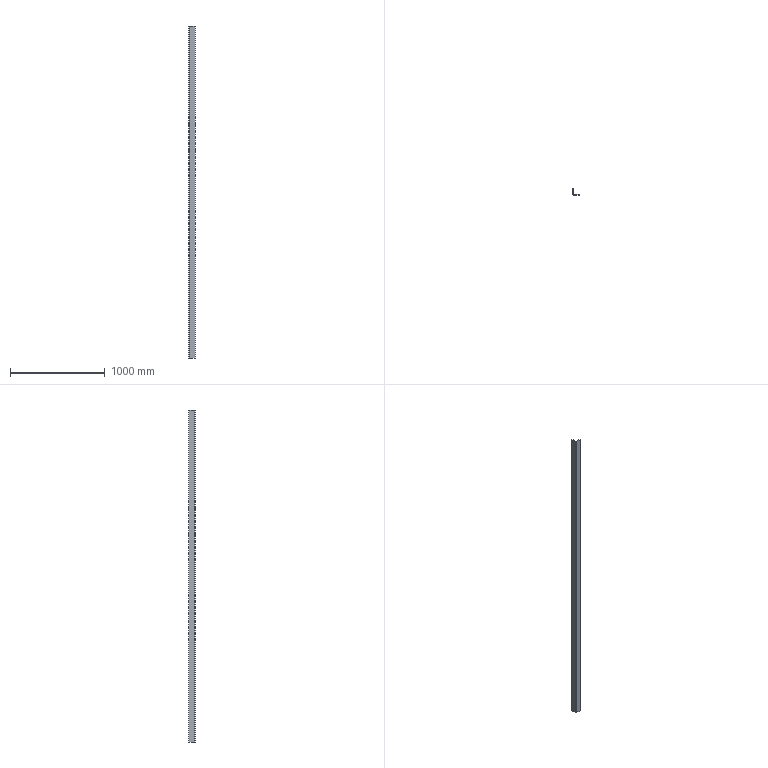Part | STEP file | BCC3 H19_8 | 1 solid | 14 faces | box 65 x 65 x 3500 mm | volume 2138678 mm3 | plane 12 | cylinder 2 | commonest cylinder face diameters 8 x1 18 x1
STEP:
#1=CARTESIAN_POINT('',(0.,0.,0.));
#2=DIRECTION('',(0.,0.,1.));
#3=DIRECTION('',(1.,0.,0.));
#4=AXIS2_PLACEMENT_3D('',#1,#2,#3);
#5=CARTESIAN_POINT('',(0.,9.,1750.));
#6=VERTEX_POINT('',#5);
#7=CARTESIAN_POINT('',(5.,9.,1750.));
#8=VERTEX_POINT('',#7);
#9=CARTESIAN_POINT('',(0.,9.,1750.));
#10=DIRECTION('',(1.,0.,0.));
#11=VECTOR('',#10,1.);
#12=LINE('',#9,#11);
#13=CARTESIAN_POINT('',(0.,9.,1750.));
#14=DIRECTION('',(0.,0.,1.));
#15=DIRECTION('',(1.,0.,0.));
#16=AXIS2_PLACEMENT_3D('',#13,#14,#15);
#17=PLANE('',#16);
#18=CARTESIAN_POINT('',(0.,0.));
#19=DIRECTION('',(1.,0.));
#20=VECTOR('',#19,1.);
#21=LINE('',#18,#20);
#22=(GEOMETRIC_REPRESENTATION_CONTEXT(2)PARAMETRIC_REPRESENTATION_CONTEXT()REPRESENTATION_CONTEXT('',''));
#23=DEFINITIONAL_REPRESENTATION('',(#21),#22);
#24=PCURVE('',#17,#23);
#25=CARTESIAN_POINT('',(9.,5.,1750.));
#26=DIRECTION('',(0.,0.,1.));
#27=DIRECTION('',(1.,0.,0.));
#28=AXIS2_PLACEMENT_3D('',#25,#26,#27);
#29=PLANE('',#28);
#30=CARTESIAN_POINT('',(-9.,4.));
#31=DIRECTION('',(1.,0.));
#32=VECTOR('',#31,1.);
#33=LINE('',#30,#32);
#34=(GEOMETRIC_REPRESENTATION_CONTEXT(2)PARAMETRIC_REPRESENTATION_CONTEXT()REPRESENTATION_CONTEXT('',''));
#35=DEFINITIONAL_REPRESENTATION('',(#33),#34);
#36=PCURVE('',#29,#35);
#37=SURFACE_CURVE('',#12,(#24,#36),.PCURVE_S1.);
#38=EDGE_CURVE('',#6,#8,#37,.T.);
#39=ORIENTED_EDGE('',*,*,#38,.F.);
#40=CARTESIAN_POINT('',(9.,0.,1750.));
#41=VERTEX_POINT('',#40);
#42=CARTESIAN_POINT('',(9.,9.,1750.));
#43=DIRECTION('',(0.,0.,1.));
#44=DIRECTION('',(-1.,0.,0.));
#45=AXIS2_PLACEMENT_3D('',#42,#43,#44);
#46=CIRCLE('',#45,9.);
#47=CARTESIAN_POINT('',(9.,0.));
#48=DIRECTION('',(-1.,0.));
#49=AXIS2_PLACEMENT_2D('',#47,#48);
#50=CIRCLE('',#49,9.);
#51=(GEOMETRIC_REPRESENTATION_CONTEXT(2)PARAMETRIC_REPRESENTATION_CONTEXT()REPRESENTATION_CONTEXT('',''));
#52=DEFINITIONAL_REPRESENTATION('',(#50),#51);
#53=PCURVE('',#17,#52);
#54=CARTESIAN_POINT('',(9.,9.,1750.));
#55=DIRECTION('',(0.,0.,-1.));
#56=DIRECTION('',(-1.,0.,0.));
#57=AXIS2_PLACEMENT_3D('',#54,#55,#56);
#58=CYLINDRICAL_SURFACE('',#57,9.);
#59=CARTESIAN_POINT('',(6.283,0.));
#60=DIRECTION('',(-1.,0.));
#61=VECTOR('',#60,1.);
#62=LINE('',#59,#61);
#63=(GEOMETRIC_REPRESENTATION_CONTEXT(2)PARAMETRIC_REPRESENTATION_CONTEXT()REPRESENTATION_CONTEXT('',''));
#64=DEFINITIONAL_REPRESENTATION('',(#62),#63);
#65=PCURVE('',#58,#64);
#66=SURFACE_CURVE('',#46,(#53,#65),.PCURVE_S1.);
#67=EDGE_CURVE('',#6,#41,#66,.T.);
#68=ORIENTED_EDGE('',*,*,#67,.T.);
#69=CARTESIAN_POINT('',(9.,5.,1750.));
#70=VERTEX_POINT('',#69);
#71=CARTESIAN_POINT('',(9.,5.,1750.));
#72=DIRECTION('',(0.,-1.,0.));
#73=VECTOR('',#72,1.);
#74=LINE('',#71,#73);
#75=CARTESIAN_POINT('',(9.,-4.));
#76=DIRECTION('',(0.,-1.));
#77=VECTOR('',#76,1.);
#78=LINE('',#75,#77);
#79=(GEOMETRIC_REPRESENTATION_CONTEXT(2)PARAMETRIC_REPRESENTATION_CONTEXT()REPRESENTATION_CONTEXT('',''));
#80=DEFINITIONAL_REPRESENTATION('',(#78),#79);
#81=PCURVE('',#17,#80);
#82=CARTESIAN_POINT('',(9.,9.,1750.));
#83=DIRECTION('',(0.,0.,1.));
#84=DIRECTION('',(1.,0.,0.));
#85=AXIS2_PLACEMENT_3D('',#82,#83,#84);
#86=PLANE('',#85);
#87=CARTESIAN_POINT('',(0.,-4.));
#88=DIRECTION('',(0.,-1.));
#89=VECTOR('',#88,1.);
#90=LINE('',#87,#89);
#91=(GEOMETRIC_REPRESENTATION_CONTEXT(2)PARAMETRIC_REPRESENTATION_CONTEXT()REPRESENTATION_CONTEXT('',''));
#92=DEFINITIONAL_REPRESENTATION('',(#90),#91);
#93=PCURVE('',#86,#92);
#94=SURFACE_CURVE('',#74,(#81,#93),.PCURVE_S1.);
#95=EDGE_CURVE('',#70,#41,#94,.T.);
#96=ORIENTED_EDGE('',*,*,#95,.F.);
#97=CARTESIAN_POINT('',(9.,9.,1750.));
#98=DIRECTION('',(0.,0.,1.));
#99=DIRECTION('',(1.,0.,0.));
#100=AXIS2_PLACEMENT_3D('',#97,#98,#99);
#101=CIRCLE('',#100,4.);
#102=CARTESIAN_POINT('',(9.,0.));
#103=DIRECTION('',(1.,0.));
#104=AXIS2_PLACEMENT_2D('',#102,#103);
#105=CIRCLE('',#104,4.);
#106=(GEOMETRIC_REPRESENTATION_CONTEXT(2)PARAMETRIC_REPRESENTATION_CONTEXT()REPRESENTATION_CONTEXT('',''));
#107=DEFINITIONAL_REPRESENTATION('',(#105),#106);
#108=PCURVE('',#17,#107);
#109=CARTESIAN_POINT('',(9.,9.,1750.));
#110=DIRECTION('',(0.,0.,-1.));
#111=DIRECTION('',(-1.,0.,0.));
#112=AXIS2_PLACEMENT_3D('',#109,#110,#111);
#113=CYLINDRICAL_SURFACE('',#112,4.);
#114=CARTESIAN_POINT('',(9.425,0.));
#115=DIRECTION('',(-1.,0.));
#116=VECTOR('',#115,1.);
#117=LINE('',#114,#116);
#118=(GEOMETRIC_REPRESENTATION_CONTEXT(2)PARAMETRIC_REPRESENTATION_CONTEXT()REPRESENTATION_CONTEXT('',''));
#119=DEFINITIONAL_REPRESENTATION('',(#117),#118);
#120=PCURVE('',#113,#119);
#121=SURFACE_CURVE('',#101,(#108,#120),.PCURVE_S1.);
#122=EDGE_CURVE('',#8,#70,#121,.T.);
#123=ORIENTED_EDGE('',*,*,#122,.F.);
#124=EDGE_LOOP('',(#39,#68,#96,#123));
#125=FACE_BOUND('',#124,.T.);
#126=ADVANCED_FACE('',(#125),#17,.T.);
#127=CARTESIAN_POINT('',(0.,65.,1750.));
#128=VERTEX_POINT('',#127);
#129=CARTESIAN_POINT('',(0.,0.,1750.));
#130=DIRECTION('',(0.,-1.,0.));
#131=VECTOR('',#130,1.);
#132=LINE('',#129,#131);
#133=CARTESIAN_POINT('',(-9.,-5.));
#134=DIRECTION('',(0.,-1.));
#135=VECTOR('',#134,1.);
#136=LINE('',#133,#135);
#137=(GEOMETRIC_REPRESENTATION_CONTEXT(2)PARAMETRIC_REPRESENTATION_CONTEXT()REPRESENTATION_CONTEXT('',''));
#138=DEFINITIONAL_REPRESENTATION('',(#136),#137);
#139=PCURVE('',#29,#138);
#140=CARTESIAN_POINT('',(0.,0.,1750.));
#141=DIRECTION('',(1.,0.,0.));
#142=DIRECTION('',(0.,0.,-1.));
#143=AXIS2_PLACEMENT_3D('',#140,#141,#142);
#144=PLANE('',#143);
#145=CARTESIAN_POINT('',(0.,0.));
#146=DIRECTION('',(0.,-1.));
#147=VECTOR('',#146,1.);
#148=LINE('',#145,#147);
#149=(GEOMETRIC_REPRESENTATION_CONTEXT(2)PARAMETRIC_REPRESENTATION_CONTEXT()REPRESENTATION_CONTEXT('',''));
#150=DEFINITIONAL_REPRESENTATION('',(#148),#149);
#151=PCURVE('',#144,#150);
#152=SURFACE_CURVE('',#132,(#139,#151),.PCURVE_S1.);
#153=EDGE_CURVE('',#128,#6,#152,.T.);
#154=ORIENTED_EDGE('',*,*,#153,.T.);
#155=ORIENTED_EDGE('',*,*,#38,.T.);
#156=CARTESIAN_POINT('',(5.,65.,1750.));
#157=VERTEX_POINT('',#156);
#158=CARTESIAN_POINT('',(5.,0.,1750.));
#159=DIRECTION('',(0.,-1.,0.));
#160=VECTOR('',#159,1.);
#161=LINE('',#158,#160);
#162=CARTESIAN_POINT('',(-4.,-5.));
#163=DIRECTION('',(0.,-1.));
#164=VECTOR('',#163,1.);
#165=LINE('',#162,#164);
#166=(GEOMETRIC_REPRESENTATION_CONTEXT(2)PARAMETRIC_REPRESENTATION_CONTEXT()REPRESENTATION_CONTEXT('',''));
#167=DEFINITIONAL_REPRESENTATION('',(#165),#166);
#168=PCURVE('',#29,#167);
#169=CARTESIAN_POINT('',(5.,0.,1750.));
#170=DIRECTION('',(1.,0.,0.));
#171=DIRECTION('',(0.,0.,-1.));
#172=AXIS2_PLACEMENT_3D('',#169,#170,#171);
#173=PLANE('',#172);
#174=CARTESIAN_POINT('',(0.,0.));
#175=DIRECTION('',(0.,-1.));
#176=VECTOR('',#175,1.);
#177=LINE('',#174,#176);
#178=(GEOMETRIC_REPRESENTATION_CONTEXT(2)PARAMETRIC_REPRESENTATION_CONTEXT()REPRESENTATION_CONTEXT('',''));
#179=DEFINITIONAL_REPRESENTATION('',(#177),#178);
#180=PCURVE('',#173,#179);
#181=SURFACE_CURVE('',#161,(#168,#180),.PCURVE_S1.);
#182=EDGE_CURVE('',#157,#8,#181,.T.);
#183=ORIENTED_EDGE('',*,*,#182,.F.);
#184=CARTESIAN_POINT('',(0.,65.,1750.));
#185=DIRECTION('',(1.,0.,0.));
#186=VECTOR('',#185,1.);
#187=LINE('',#184,#186);
#188=CARTESIAN_POINT('',(-9.,60.));
#189=DIRECTION('',(1.,0.));
#190=VECTOR('',#189,1.);
#191=LINE('',#188,#190);
#192=(GEOMETRIC_REPRESENTATION_CONTEXT(2)PARAMETRIC_REPRESENTATION_CONTEXT()REPRESENTATION_CONTEXT('',''));
#193=DEFINITIONAL_REPRESENTATION('',(#191),#192);
#194=PCURVE('',#29,#193);
#195=CARTESIAN_POINT('',(0.,65.,1750.));
#196=DIRECTION('',(0.,1.,0.));
#197=DIRECTION('',(0.,0.,1.));
#198=AXIS2_PLACEMENT_3D('',#195,#196,#197);
#199=PLANE('',#198);
#200=CARTESIAN_POINT('',(0.,0.));
#201=DIRECTION('',(0.,1.));
#202=VECTOR('',#201,1.);
#203=LINE('',#200,#202);
#204=(GEOMETRIC_REPRESENTATION_CONTEXT(2)PARAMETRIC_REPRESENTATION_CONTEXT()REPRESENTATION_CONTEXT('',''));
#205=DEFINITIONAL_REPRESENTATION('',(#203),#204);
#206=PCURVE('',#199,#205);
#207=SURFACE_CURVE('',#187,(#194,#206),.PCURVE_S1.);
#208=EDGE_CURVE('',#128,#157,#207,.T.);
#209=ORIENTED_EDGE('',*,*,#208,.F.);
#210=EDGE_LOOP('',(#154,#155,#183,#209));
#211=FACE_BOUND('',#210,.T.);
#212=ADVANCED_FACE('',(#211),#29,.T.);
#213=CARTESIAN_POINT('',(9.,0.,-1750.));
#214=VERTEX_POINT('',#213);
#215=CARTESIAN_POINT('',(9.,5.,-1750.));
#216=VERTEX_POINT('',#215);
#217=CARTESIAN_POINT('',(9.,0.,-1750.));
#218=DIRECTION('',(0.,1.,0.));
#219=VECTOR('',#218,1.);
#220=LINE('',#217,#219);
#221=CARTESIAN_POINT('',(9.,0.,-1750.));
#222=DIRECTION('',(0.,0.,-1.));
#223=DIRECTION('',(-1.,0.,0.));
#224=AXIS2_PLACEMENT_3D('',#221,#222,#223);
#225=PLANE('',#224);
#226=CARTESIAN_POINT('',(0.,0.));
#227=DIRECTION('',(0.,1.));
#228=VECTOR('',#227,1.);
#229=LINE('',#226,#228);
#230=(GEOMETRIC_REPRESENTATION_CONTEXT(2)PARAMETRIC_REPRESENTATION_CONTEXT()REPRESENTATION_CONTEXT('',''));
#231=DEFINITIONAL_REPRESENTATION('',(#229),#230);
#232=PCURVE('',#225,#231);
#233=CARTESIAN_POINT('',(5.,9.,-1750.));
#234=DIRECTION('',(0.,0.,-1.));
#235=DIRECTION('',(-1.,0.,0.));
#236=AXIS2_PLACEMENT_3D('',#233,#234,#235);
#237=PLANE('',#236);
#238=CARTESIAN_POINT('',(-4.,-9.));
#239=DIRECTION('',(0.,1.));
#240=VECTOR('',#239,1.);
#241=LINE('',#238,#240);
#242=(GEOMETRIC_REPRESENTATION_CONTEXT(2)PARAMETRIC_REPRESENTATION_CONTEXT()REPRESENTATION_CONTEXT('',''));
#243=DEFINITIONAL_REPRESENTATION('',(#241),#242);
#244=PCURVE('',#237,#243);
#245=SURFACE_CURVE('',#220,(#232,#244),.PCURVE_S1.);
#246=EDGE_CURVE('',#214,#216,#245,.T.);
#247=ORIENTED_EDGE('',*,*,#246,.F.);
#248=CARTESIAN_POINT('',(0.,9.,-1750.));
#249=VERTEX_POINT('',#248);
#250=CARTESIAN_POINT('',(9.,9.,-1750.));
#251=DIRECTION('',(0.,0.,1.));
#252=DIRECTION('',(-1.,0.,0.));
#253=AXIS2_PLACEMENT_3D('',#250,#251,#252);
#254=CIRCLE('',#253,9.);
#255=CARTESIAN_POINT('',(9.,9.));
#256=CARTESIAN_POINT('',(9.,-6.588));
#257=CARTESIAN_POINT('',(-4.5,1.206));
#258=CARTESIAN_POINT('',(-18.,9.));
#259=CARTESIAN_POINT('',(-4.5,16.794));
#260=CARTESIAN_POINT('',(9.,24.588));
#261=CARTESIAN_POINT('',(9.,9.));
#262=(BOUNDED_CURVE()B_SPLINE_CURVE(2,(#255,#256,#257,#258,#259,#260,#261),.UNSPECIFIED.,.T.,.F.)B_SPLINE_CURVE_WITH_KNOTS((1,2,2,2,2,1),(-2.094,0.,2.094,4.189,6.283,8.378),.UNSPECIFIED.)CURVE()GEOMETRIC_REPRESENTATION_ITEM()RATIONAL_B_SPLINE_CURVE((1.,0.5,1.,0.5,1.,0.5,1.))REPRESENTATION_ITEM(''));
#263=(GEOMETRIC_REPRESENTATION_CONTEXT(2)PARAMETRIC_REPRESENTATION_CONTEXT()REPRESENTATION_CONTEXT('',''));
#264=DEFINITIONAL_REPRESENTATION('',(#262),#263);
#265=PCURVE('',#225,#264);
#266=CARTESIAN_POINT('',(6.283,3500.));
#267=DIRECTION('',(-1.,0.));
#268=VECTOR('',#267,1.);
#269=LINE('',#266,#268);
#270=(GEOMETRIC_REPRESENTATION_CONTEXT(2)PARAMETRIC_REPRESENTATION_CONTEXT()REPRESENTATION_CONTEXT('',''));
#271=DEFINITIONAL_REPRESENTATION('',(#269),#270);
#272=PCURVE('',#58,#271);
#273=SURFACE_CURVE('',#254,(#265,#272),.PCURVE_S1.);
#274=EDGE_CURVE('',#249,#214,#273,.T.);
#275=ORIENTED_EDGE('',*,*,#274,.F.);
#276=CARTESIAN_POINT('',(5.,9.,-1750.));
#277=VERTEX_POINT('',#276);
#278=CARTESIAN_POINT('',(5.,9.,-1750.));
#279=DIRECTION('',(-1.,0.,0.));
#280=VECTOR('',#279,1.);
#281=LINE('',#278,#280);
#282=CARTESIAN_POINT('',(4.,9.));
#283=DIRECTION('',(1.,0.));
#284=VECTOR('',#283,1.);
#285=LINE('',#282,#284);
#286=(GEOMETRIC_REPRESENTATION_CONTEXT(2)PARAMETRIC_REPRESENTATION_CONTEXT()REPRESENTATION_CONTEXT('',''));
#287=DEFINITIONAL_REPRESENTATION('',(#285),#286);
#288=PCURVE('',#225,#287);
#289=CARTESIAN_POINT('',(9.,9.,-1750.));
#290=DIRECTION('',(0.,0.,1.));
#291=DIRECTION('',(1.,0.,0.));
#292=AXIS2_PLACEMENT_3D('',#289,#290,#291);
#293=PLANE('',#292);
#294=CARTESIAN_POINT('',(-4.,0.));
#295=DIRECTION('',(-1.,0.));
#296=VECTOR('',#295,1.);
#297=LINE('',#294,#296);
#298=(GEOMETRIC_REPRESENTATION_CONTEXT(2)PARAMETRIC_REPRESENTATION_CONTEXT()REPRESENTATION_CONTEXT('',''));
#299=DEFINITIONAL_REPRESENTATION('',(#297),#298);
#300=PCURVE('',#293,#299);
#301=SURFACE_CURVE('',#281,(#288,#300),.PCURVE_S1.);
#302=EDGE_CURVE('',#277,#249,#301,.T.);
#303=ORIENTED_EDGE('',*,*,#302,.F.);
#304=CARTESIAN_POINT('',(9.,9.,-1750.));
#305=DIRECTION('',(0.,0.,1.));
#306=DIRECTION('',(1.,0.,0.));
#307=AXIS2_PLACEMENT_3D('',#304,#305,#306);
#308=CIRCLE('',#307,4.);
#309=CARTESIAN_POINT('',(-4.,9.));
#310=CARTESIAN_POINT('',(-4.,15.928));
#311=CARTESIAN_POINT('',(2.,12.464));
#312=CARTESIAN_POINT('',(8.,9.));
#313=CARTESIAN_POINT('',(2.,5.536));
#314=CARTESIAN_POINT('',(-4.,2.072));
#315=CARTESIAN_POINT('',(-4.,9.));
#316=(BOUNDED_CURVE()B_SPLINE_CURVE(2,(#309,#310,#311,#312,#313,#314,#315),.UNSPECIFIED.,.T.,.F.)B_SPLINE_CURVE_WITH_KNOTS((1,2,2,2,2,1),(-2.094,0.,2.094,4.189,6.283,8.378),.UNSPECIFIED.)CURVE()GEOMETRIC_REPRESENTATION_ITEM()RATIONAL_B_SPLINE_CURVE((1.,0.5,1.,0.5,1.,0.5,1.))REPRESENTATION_ITEM(''));
#317=(GEOMETRIC_REPRESENTATION_CONTEXT(2)PARAMETRIC_REPRESENTATION_CONTEXT()REPRESENTATION_CONTEXT('',''));
#318=DEFINITIONAL_REPRESENTATION('',(#316),#317);
#319=PCURVE('',#225,#318);
#320=CARTESIAN_POINT('',(9.425,3500.));
#321=DIRECTION('',(-1.,0.));
#322=VECTOR('',#321,1.);
#323=LINE('',#320,#322);
#324=(GEOMETRIC_REPRESENTATION_CONTEXT(2)PARAMETRIC_REPRESENTATION_CONTEXT()REPRESENTATION_CONTEXT('',''));
#325=DEFINITIONAL_REPRESENTATION('',(#323),#324);
#326=PCURVE('',#113,#325);
#327=SURFACE_CURVE('',#308,(#319,#326),.PCURVE_S1.);
#328=EDGE_CURVE('',#277,#216,#327,.T.);
#329=ORIENTED_EDGE('',*,*,#328,.T.);
#330=EDGE_LOOP('',(#247,#275,#303,#329));
#331=FACE_BOUND('',#330,.T.);
#332=ADVANCED_FACE('',(#331),#225,.T.);
#333=CARTESIAN_POINT('',(65.,0.,-1750.));
#334=VERTEX_POINT('',#333);
#335=CARTESIAN_POINT('',(0.,0.,-1750.));
#336=DIRECTION('',(1.,0.,0.));
#337=VECTOR('',#336,1.);
#338=LINE('',#335,#337);
#339=CARTESIAN_POINT('',(5.,-9.));
#340=DIRECTION('',(-1.,0.));
#341=VECTOR('',#340,1.);
#342=LINE('',#339,#341);
#343=(GEOMETRIC_REPRESENTATION_CONTEXT(2)PARAMETRIC_REPRESENTATION_CONTEXT()REPRESENTATION_CONTEXT('',''));
#344=DEFINITIONAL_REPRESENTATION('',(#342),#343);
#345=PCURVE('',#237,#344);
#346=CARTESIAN_POINT('',(0.,0.,1750.));
#347=DIRECTION('',(0.,1.,0.));
#348=DIRECTION('',(0.,0.,1.));
#349=AXIS2_PLACEMENT_3D('',#346,#347,#348);
#350=PLANE('',#349);
#351=CARTESIAN_POINT('',(-3500.,0.));
#352=DIRECTION('',(0.,1.));
#353=VECTOR('',#352,1.);
#354=LINE('',#351,#353);
#355=(GEOMETRIC_REPRESENTATION_CONTEXT(2)PARAMETRIC_REPRESENTATION_CONTEXT()REPRESENTATION_CONTEXT('',''));
#356=DEFINITIONAL_REPRESENTATION('',(#354),#355);
#357=PCURVE('',#350,#356);
#358=SURFACE_CURVE('',#338,(#345,#357),.PCURVE_S1.);
#359=EDGE_CURVE('',#214,#334,#358,.T.);
#360=ORIENTED_EDGE('',*,*,#359,.F.);
#361=ORIENTED_EDGE('',*,*,#246,.T.);
#362=CARTESIAN_POINT('',(65.,5.,-1750.));
#363=VERTEX_POINT('',#362);
#364=CARTESIAN_POINT('',(0.,5.,-1750.));
#365=DIRECTION('',(1.,0.,0.));
#366=VECTOR('',#365,1.);
#367=LINE('',#364,#366);
#368=CARTESIAN_POINT('',(5.,-4.));
#369=DIRECTION('',(-1.,0.));
#370=VECTOR('',#369,1.);
#371=LINE('',#368,#370);
#372=(GEOMETRIC_REPRESENTATION_CONTEXT(2)PARAMETRIC_REPRESENTATION_CONTEXT()REPRESENTATION_CONTEXT('',''));
#373=DEFINITIONAL_REPRESENTATION('',(#371),#372);
#374=PCURVE('',#237,#373);
#375=CARTESIAN_POINT('',(0.,5.,1750.));
#376=DIRECTION('',(0.,1.,0.));
#377=DIRECTION('',(0.,0.,1.));
#378=AXIS2_PLACEMENT_3D('',#375,#376,#377);
#379=PLANE('',#378);
#380=CARTESIAN_POINT('',(-3500.,0.));
#381=DIRECTION('',(0.,1.));
#382=VECTOR('',#381,1.);
#383=LINE('',#380,#382);
#384=(GEOMETRIC_REPRESENTATION_CONTEXT(2)PARAMETRIC_REPRESENTATION_CONTEXT()REPRESENTATION_CONTEXT('',''));
#385=DEFINITIONAL_REPRESENTATION('',(#383),#384);
#386=PCURVE('',#379,#385);
#387=SURFACE_CURVE('',#367,(#374,#386),.PCURVE_S1.);
#388=EDGE_CURVE('',#216,#363,#387,.T.);
#389=ORIENTED_EDGE('',*,*,#388,.T.);
#390=CARTESIAN_POINT('',(65.,5.,-1750.));
#391=DIRECTION('',(0.,-1.,0.));
#392=VECTOR('',#391,1.);
#393=LINE('',#390,#392);
#394=CARTESIAN_POINT('',(-60.,-4.));
#395=DIRECTION('',(0.,-1.));
#396=VECTOR('',#395,1.);
#397=LINE('',#394,#396);
#398=(GEOMETRIC_REPRESENTATION_CONTEXT(2)PARAMETRIC_REPRESENTATION_CONTEXT()REPRESENTATION_CONTEXT('',''));
#399=DEFINITIONAL_REPRESENTATION('',(#397),#398);
#400=PCURVE('',#237,#399);
#401=CARTESIAN_POINT('',(65.,5.,1750.));
#402=DIRECTION('',(1.,0.,0.));
#403=DIRECTION('',(0.,0.,-1.));
#404=AXIS2_PLACEMENT_3D('',#401,#402,#403);
#405=PLANE('',#404);
#406=CARTESIAN_POINT('',(3500.,0.));
#407=DIRECTION('',(0.,-1.));
#408=VECTOR('',#407,1.);
#409=LINE('',#406,#408);
#410=(GEOMETRIC_REPRESENTATION_CONTEXT(2)PARAMETRIC_REPRESENTATION_CONTEXT()REPRESENTATION_CONTEXT('',''));
#411=DEFINITIONAL_REPRESENTATION('',(#409),#410);
#412=PCURVE('',#405,#411);
#413=SURFACE_CURVE('',#393,(#400,#412),.PCURVE_S1.);
#414=EDGE_CURVE('',#363,#334,#413,.T.);
#415=ORIENTED_EDGE('',*,*,#414,.T.);
#416=EDGE_LOOP('',(#360,#361,#389,#415));
#417=FACE_BOUND('',#416,.T.);
#418=ADVANCED_FACE('',(#417),#237,.T.);
#419=ORIENTED_EDGE('',*,*,#359,.T.);
#420=CARTESIAN_POINT('',(65.,0.,1750.));
#421=VERTEX_POINT('',#420);
#422=CARTESIAN_POINT('',(65.,0.,1750.));
#423=DIRECTION('',(0.,0.,-1.));
#424=VECTOR('',#423,1.);
#425=LINE('',#422,#424);
#426=CARTESIAN_POINT('',(0.,65.));
#427=DIRECTION('',(-1.,0.));
#428=VECTOR('',#427,1.);
#429=LINE('',#426,#428);
#430=(GEOMETRIC_REPRESENTATION_CONTEXT(2)PARAMETRIC_REPRESENTATION_CONTEXT()REPRESENTATION_CONTEXT('',''));
#431=DEFINITIONAL_REPRESENTATION('',(#429),#430);
#432=PCURVE('',#350,#431);
#433=CARTESIAN_POINT('',(0.,-5.));
#434=DIRECTION('',(1.,0.));
#435=VECTOR('',#434,1.);
#436=LINE('',#433,#435);
#437=(GEOMETRIC_REPRESENTATION_CONTEXT(2)PARAMETRIC_REPRESENTATION_CONTEXT()REPRESENTATION_CONTEXT('',''));
#438=DEFINITIONAL_REPRESENTATION('',(#436),#437);
#439=PCURVE('',#405,#438);
#440=SURFACE_CURVE('',#425,(#432,#439),.PCURVE_S1.);
#441=EDGE_CURVE('',#421,#334,#440,.T.);
#442=ORIENTED_EDGE('',*,*,#441,.F.);
#443=CARTESIAN_POINT('',(0.,0.,1750.));
#444=DIRECTION('',(1.,0.,0.));
#445=VECTOR('',#444,1.);
#446=LINE('',#443,#445);
#447=CARTESIAN_POINT('',(0.,0.));
#448=DIRECTION('',(0.,1.));
#449=VECTOR('',#448,1.);
#450=LINE('',#447,#449);
#451=(GEOMETRIC_REPRESENTATION_CONTEXT(2)PARAMETRIC_REPRESENTATION_CONTEXT()REPRESENTATION_CONTEXT('',''));
#452=DEFINITIONAL_REPRESENTATION('',(#450),#451);
#453=PCURVE('',#350,#452);
#454=CARTESIAN_POINT('',(-9.,-9.));
#455=DIRECTION('',(1.,0.));
#456=VECTOR('',#455,1.);
#457=LINE('',#454,#456);
#458=(GEOMETRIC_REPRESENTATION_CONTEXT(2)PARAMETRIC_REPRESENTATION_CONTEXT()REPRESENTATION_CONTEXT('',''));
#459=DEFINITIONAL_REPRESENTATION('',(#457),#458);
#460=PCURVE('',#86,#459);
#461=SURFACE_CURVE('',#446,(#453,#460),.PCURVE_S1.);
#462=EDGE_CURVE('',#41,#421,#461,.T.);
#463=ORIENTED_EDGE('',*,*,#462,.F.);
#464=CARTESIAN_POINT('',(9.,0.,1750.));
#465=DIRECTION('',(0.,0.,-1.));
#466=VECTOR('',#465,1.);
#467=LINE('',#464,#466);
#468=CARTESIAN_POINT('',(0.,9.));
#469=DIRECTION('',(-1.,0.));
#470=VECTOR('',#469,1.);
#471=LINE('',#468,#470);
#472=(GEOMETRIC_REPRESENTATION_CONTEXT(2)PARAMETRIC_REPRESENTATION_CONTEXT()REPRESENTATION_CONTEXT('',''));
#473=DEFINITIONAL_REPRESENTATION('',(#471),#472);
#474=PCURVE('',#350,#473);
#475=CARTESIAN_POINT('',(4.712,0.));
#476=DIRECTION('',(0.,1.));
#477=VECTOR('',#476,1.);
#478=LINE('',#475,#477);
#479=(GEOMETRIC_REPRESENTATION_CONTEXT(2)PARAMETRIC_REPRESENTATION_CONTEXT()REPRESENTATION_CONTEXT('',''));
#480=DEFINITIONAL_REPRESENTATION('',(#478),#479);
#481=PCURVE('',#58,#480);
#482=SURFACE_CURVE('',#467,(#474,#481),.PCURVE_S1.);
#483=EDGE_CURVE('',#41,#214,#482,.T.);
#484=ORIENTED_EDGE('',*,*,#483,.T.);
#485=EDGE_LOOP('',(#419,#442,#463,#484));
#486=FACE_BOUND('',#485,.T.);
#487=ADVANCED_FACE('',(#486),#350,.F.);
#488=ORIENTED_EDGE('',*,*,#414,.F.);
#489=CARTESIAN_POINT('',(65.,5.,1750.));
#490=VERTEX_POINT('',#489);
#491=CARTESIAN_POINT('',(65.,5.,1750.));
#492=DIRECTION('',(0.,0.,-1.));
#493=VECTOR('',#492,1.);
#494=LINE('',#491,#493);
#495=CARTESIAN_POINT('',(0.,0.));
#496=DIRECTION('',(1.,0.));
#497=VECTOR('',#496,1.);
#498=LINE('',#495,#497);
#499=(GEOMETRIC_REPRESENTATION_CONTEXT(2)PARAMETRIC_REPRESENTATION_CONTEXT()REPRESENTATION_CONTEXT('',''));
#500=DEFINITIONAL_REPRESENTATION('',(#498),#499);
#501=PCURVE('',#405,#500);
#502=CARTESIAN_POINT('',(0.,65.));
#503=DIRECTION('',(-1.,0.));
#504=VECTOR('',#503,1.);
#505=LINE('',#502,#504);
#506=(GEOMETRIC_REPRESENTATION_CONTEXT(2)PARAMETRIC_REPRESENTATION_CONTEXT()REPRESENTATION_CONTEXT('',''));
#507=DEFINITIONAL_REPRESENTATION('',(#505),#506);
#508=PCURVE('',#379,#507);
#509=SURFACE_CURVE('',#494,(#501,#508),.PCURVE_S1.);
#510=EDGE_CURVE('',#490,#363,#509,.T.);
#511=ORIENTED_EDGE('',*,*,#510,.F.);
#512=CARTESIAN_POINT('',(65.,5.,1750.));
#513=DIRECTION('',(0.,-1.,0.));
#514=VECTOR('',#513,1.);
#515=LINE('',#512,#514);
#516=CARTESIAN_POINT('',(0.,0.));
#517=DIRECTION('',(0.,-1.));
#518=VECTOR('',#517,1.);
#519=LINE('',#516,#518);
#520=(GEOMETRIC_REPRESENTATION_CONTEXT(2)PARAMETRIC_REPRESENTATION_CONTEXT()REPRESENTATION_CONTEXT('',''));
#521=DEFINITIONAL_REPRESENTATION('',(#519),#520);
#522=PCURVE('',#405,#521);
#523=CARTESIAN_POINT('',(56.,-4.));
#524=DIRECTION('',(0.,-1.));
#525=VECTOR('',#524,1.);
#526=LINE('',#523,#525);
#527=(GEOMETRIC_REPRESENTATION_CONTEXT(2)PARAMETRIC_REPRESENTATION_CONTEXT()REPRESENTATION_CONTEXT('',''));
#528=DEFINITIONAL_REPRESENTATION('',(#526),#527);
#529=PCURVE('',#86,#528);
#530=SURFACE_CURVE('',#515,(#522,#529),.PCURVE_S1.);
#531=EDGE_CURVE('',#490,#421,#530,.T.);
#532=ORIENTED_EDGE('',*,*,#531,.T.);
#533=ORIENTED_EDGE('',*,*,#441,.T.);
#534=EDGE_LOOP('',(#488,#511,#532,#533));
#535=FACE_BOUND('',#534,.T.);
#536=ADVANCED_FACE('',(#535),#405,.T.);
#537=ORIENTED_EDGE('',*,*,#388,.F.);
#538=CARTESIAN_POINT('',(9.,5.,1750.));
#539=DIRECTION('',(0.,0.,-1.));
#540=VECTOR('',#539,1.);
#541=LINE('',#538,#540);
#542=CARTESIAN_POINT('',(0.,9.));
#543=DIRECTION('',(-1.,0.));
#544=VECTOR('',#543,1.);
#545=LINE('',#542,#544);
#546=(GEOMETRIC_REPRESENTATION_CONTEXT(2)PARAMETRIC_REPRESENTATION_CONTEXT()REPRESENTATION_CONTEXT('',''));
#547=DEFINITIONAL_REPRESENTATION('',(#545),#546);
#548=PCURVE('',#379,#547);
#549=CARTESIAN_POINT('',(4.712,0.));
#550=DIRECTION('',(0.,1.));
#551=VECTOR('',#550,1.);
#552=LINE('',#549,#551);
#553=(GEOMETRIC_REPRESENTATION_CONTEXT(2)PARAMETRIC_REPRESENTATION_CONTEXT()REPRESENTATION_CONTEXT('',''));
#554=DEFINITIONAL_REPRESENTATION('',(#552),#553);
#555=PCURVE('',#113,#554);
#556=SURFACE_CURVE('',#541,(#548,#555),.PCURVE_S1.);
#557=EDGE_CURVE('',#70,#216,#556,.T.);
#558=ORIENTED_EDGE('',*,*,#557,.F.);
#559=CARTESIAN_POINT('',(0.,5.,1750.));
#560=DIRECTION('',(1.,0.,0.));
#561=VECTOR('',#560,1.);
#562=LINE('',#559,#561);
#563=CARTESIAN_POINT('',(0.,0.));
#564=DIRECTION('',(0.,1.));
#565=VECTOR('',#564,1.);
#566=LINE('',#563,#565);
#567=(GEOMETRIC_REPRESENTATION_CONTEXT(2)PARAMETRIC_REPRESENTATION_CONTEXT()REPRESENTATION_CONTEXT('',''));
#568=DEFINITIONAL_REPRESENTATION('',(#566),#567);
#569=PCURVE('',#379,#568);
#570=CARTESIAN_POINT('',(-9.,-4.));
#571=DIRECTION('',(1.,0.));
#572=VECTOR('',#571,1.);
#573=LINE('',#570,#572);
#574=(GEOMETRIC_REPRESENTATION_CONTEXT(2)PARAMETRIC_REPRESENTATION_CONTEXT()REPRESENTATION_CONTEXT('',''));
#575=DEFINITIONAL_REPRESENTATION('',(#573),#574);
#576=PCURVE('',#86,#575);
#577=SURFACE_CURVE('',#562,(#569,#576),.PCURVE_S1.);
#578=EDGE_CURVE('',#70,#490,#577,.T.);
#579=ORIENTED_EDGE('',*,*,#578,.T.);
#580=ORIENTED_EDGE('',*,*,#510,.T.);
#581=EDGE_LOOP('',(#537,#558,#579,#580));
#582=FACE_BOUND('',#581,.T.);
#583=ADVANCED_FACE('',(#582),#379,.T.);
#584=ORIENTED_EDGE('',*,*,#557,.F.);
#585=ORIENTED_EDGE('',*,*,#122,.F.);
#586=CARTESIAN_POINT('',(5.,9.,1750.));
#587=DIRECTION('',(0.,0.,-1.));
#588=VECTOR('',#587,1.);
#589=LINE('',#586,#588);
#590=CARTESIAN_POINT('',(6.283,0.));
#591=DIRECTION('',(0.,1.));
#592=VECTOR('',#591,1.);
#593=LINE('',#590,#592);
#594=(GEOMETRIC_REPRESENTATION_CONTEXT(2)PARAMETRIC_REPRESENTATION_CONTEXT()REPRESENTATION_CONTEXT('',''));
#595=DEFINITIONAL_REPRESENTATION('',(#593),#594);
#596=PCURVE('',#113,#595);
#597=CARTESIAN_POINT('',(0.,9.));
#598=DIRECTION('',(1.,0.));
#599=VECTOR('',#598,1.);
#600=LINE('',#597,#599);
#601=(GEOMETRIC_REPRESENTATION_CONTEXT(2)PARAMETRIC_REPRESENTATION_CONTEXT()REPRESENTATION_CONTEXT('',''));
#602=DEFINITIONAL_REPRESENTATION('',(#600),#601);
#603=PCURVE('',#173,#602);
#604=SURFACE_CURVE('',#589,(#596,#603),.PCURVE_S1.);
#605=EDGE_CURVE('',#8,#277,#604,.T.);
#606=ORIENTED_EDGE('',*,*,#605,.T.);
#607=ORIENTED_EDGE('',*,*,#328,.T.);
#608=EDGE_LOOP('',(#584,#585,#606,#607));
#609=FACE_BOUND('',#608,.F.);
#610=ADVANCED_FACE('',(#609),#113,.F.);
#611=CARTESIAN_POINT('',(5.,65.,-1750.));
#612=VERTEX_POINT('',#611);
#613=CARTESIAN_POINT('',(5.,0.,-1750.));
#614=DIRECTION('',(0.,-1.,0.));
#615=VECTOR('',#614,1.);
#616=LINE('',#613,#615);
#617=CARTESIAN_POINT('',(3500.,0.));
#618=DIRECTION('',(0.,-1.));
#619=VECTOR('',#618,1.);
#620=LINE('',#617,#619);
#621=(GEOMETRIC_REPRESENTATION_CONTEXT(2)PARAMETRIC_REPRESENTATION_CONTEXT()REPRESENTATION_CONTEXT('',''));
#622=DEFINITIONAL_REPRESENTATION('',(#620),#621);
#623=PCURVE('',#173,#622);
#624=CARTESIAN_POINT('',(-4.,-9.));
#625=DIRECTION('',(0.,-1.));
#626=VECTOR('',#625,1.);
#627=LINE('',#624,#626);
#628=(GEOMETRIC_REPRESENTATION_CONTEXT(2)PARAMETRIC_REPRESENTATION_CONTEXT()REPRESENTATION_CONTEXT('',''));
#629=DEFINITIONAL_REPRESENTATION('',(#627),#628);
#630=PCURVE('',#293,#629);
#631=SURFACE_CURVE('',#616,(#623,#630),.PCURVE_S1.);
#632=EDGE_CURVE('',#612,#277,#631,.T.);
#633=ORIENTED_EDGE('',*,*,#632,.F.);
#634=CARTESIAN_POINT('',(5.,65.,1750.));
#635=DIRECTION('',(0.,0.,-1.));
#636=VECTOR('',#635,1.);
#637=LINE('',#634,#636);
#638=CARTESIAN_POINT('',(0.,65.));
#639=DIRECTION('',(1.,0.));
#640=VECTOR('',#639,1.);
#641=LINE('',#638,#640);
#642=(GEOMETRIC_REPRESENTATION_CONTEXT(2)PARAMETRIC_REPRESENTATION_CONTEXT()REPRESENTATION_CONTEXT('',''));
#643=DEFINITIONAL_REPRESENTATION('',(#641),#642);
#644=PCURVE('',#173,#643);
#645=CARTESIAN_POINT('',(0.,5.));
#646=DIRECTION('',(-1.,0.));
#647=VECTOR('',#646,1.);
#648=LINE('',#645,#647);
#649=(GEOMETRIC_REPRESENTATION_CONTEXT(2)PARAMETRIC_REPRESENTATION_CONTEXT()REPRESENTATION_CONTEXT('',''));
#650=DEFINITIONAL_REPRESENTATION('',(#648),#649);
#651=PCURVE('',#199,#650);
#652=SURFACE_CURVE('',#637,(#644,#651),.PCURVE_S1.);
#653=EDGE_CURVE('',#157,#612,#652,.T.);
#654=ORIENTED_EDGE('',*,*,#653,.F.);
#655=ORIENTED_EDGE('',*,*,#182,.T.);
#656=ORIENTED_EDGE('',*,*,#605,.T.);
#657=EDGE_LOOP('',(#633,#654,#655,#656));
#658=FACE_BOUND('',#657,.T.);
#659=ADVANCED_FACE('',(#658),#173,.T.);
#660=CARTESIAN_POINT('',(0.,65.,-1750.));
#661=VERTEX_POINT('',#660);
#662=CARTESIAN_POINT('',(0.,65.,-1750.));
#663=DIRECTION('',(1.,0.,0.));
#664=VECTOR('',#663,1.);
#665=LINE('',#662,#664);
#666=CARTESIAN_POINT('',(-3500.,0.));
#667=DIRECTION('',(0.,1.));
#668=VECTOR('',#667,1.);
#669=LINE('',#666,#668);
#670=(GEOMETRIC_REPRESENTATION_CONTEXT(2)PARAMETRIC_REPRESENTATION_CONTEXT()REPRESENTATION_CONTEXT('',''));
#671=DEFINITIONAL_REPRESENTATION('',(#669),#670);
#672=PCURVE('',#199,#671);
#673=CARTESIAN_POINT('',(-9.,56.));
#674=DIRECTION('',(1.,0.));
#675=VECTOR('',#674,1.);
#676=LINE('',#673,#675);
#677=(GEOMETRIC_REPRESENTATION_CONTEXT(2)PARAMETRIC_REPRESENTATION_CONTEXT()REPRESENTATION_CONTEXT('',''));
#678=DEFINITIONAL_REPRESENTATION('',(#676),#677);
#679=PCURVE('',#293,#678);
#680=SURFACE_CURVE('',#665,(#672,#679),.PCURVE_S1.);
#681=EDGE_CURVE('',#661,#612,#680,.T.);
#682=ORIENTED_EDGE('',*,*,#681,.F.);
#683=CARTESIAN_POINT('',(0.,65.,1750.));
#684=DIRECTION('',(0.,0.,-1.));
#685=VECTOR('',#684,1.);
#686=LINE('',#683,#685);
#687=CARTESIAN_POINT('',(0.,0.));
#688=DIRECTION('',(-1.,0.));
#689=VECTOR('',#688,1.);
#690=LINE('',#687,#689);
#691=(GEOMETRIC_REPRESENTATION_CONTEXT(2)PARAMETRIC_REPRESENTATION_CONTEXT()REPRESENTATION_CONTEXT('',''));
#692=DEFINITIONAL_REPRESENTATION('',(#690),#691);
#693=PCURVE('',#199,#692);
#694=CARTESIAN_POINT('',(0.,65.));
#695=DIRECTION('',(1.,0.));
#696=VECTOR('',#695,1.);
#697=LINE('',#694,#696);
#698=(GEOMETRIC_REPRESENTATION_CONTEXT(2)PARAMETRIC_REPRESENTATION_CONTEXT()REPRESENTATION_CONTEXT('',''));
#699=DEFINITIONAL_REPRESENTATION('',(#697),#698);
#700=PCURVE('',#144,#699);
#701=SURFACE_CURVE('',#686,(#693,#700),.PCURVE_S1.);
#702=EDGE_CURVE('',#128,#661,#701,.T.);
#703=ORIENTED_EDGE('',*,*,#702,.F.);
#704=ORIENTED_EDGE('',*,*,#208,.T.);
#705=ORIENTED_EDGE('',*,*,#653,.T.);
#706=EDGE_LOOP('',(#682,#703,#704,#705));
#707=FACE_BOUND('',#706,.T.);
#708=ADVANCED_FACE('',(#707),#199,.T.);
#709=CARTESIAN_POINT('',(0.,0.,-1750.));
#710=DIRECTION('',(0.,-1.,0.));
#711=VECTOR('',#710,1.);
#712=LINE('',#709,#711);
#713=CARTESIAN_POINT('',(3500.,0.));
#714=DIRECTION('',(0.,-1.));
#715=VECTOR('',#714,1.);
#716=LINE('',#713,#715);
#717=(GEOMETRIC_REPRESENTATION_CONTEXT(2)PARAMETRIC_REPRESENTATION_CONTEXT()REPRESENTATION_CONTEXT('',''));
#718=DEFINITIONAL_REPRESENTATION('',(#716),#717);
#719=PCURVE('',#144,#718);
#720=CARTESIAN_POINT('',(-9.,-9.));
#721=DIRECTION('',(0.,-1.));
#722=VECTOR('',#721,1.);
#723=LINE('',#720,#722);
#724=(GEOMETRIC_REPRESENTATION_CONTEXT(2)PARAMETRIC_REPRESENTATION_CONTEXT()REPRESENTATION_CONTEXT('',''));
#725=DEFINITIONAL_REPRESENTATION('',(#723),#724);
#726=PCURVE('',#293,#725);
#727=SURFACE_CURVE('',#712,(#719,#726),.PCURVE_S1.);
#728=EDGE_CURVE('',#661,#249,#727,.T.);
#729=ORIENTED_EDGE('',*,*,#728,.T.);
#730=CARTESIAN_POINT('',(0.,9.,1750.));
#731=DIRECTION('',(0.,0.,-1.));
#732=VECTOR('',#731,1.);
#733=LINE('',#730,#732);
#734=CARTESIAN_POINT('',(0.,9.));
#735=DIRECTION('',(1.,0.));
#736=VECTOR('',#735,1.);
#737=LINE('',#734,#736);
#738=(GEOMETRIC_REPRESENTATION_CONTEXT(2)PARAMETRIC_REPRESENTATION_CONTEXT()REPRESENTATION_CONTEXT('',''));
#739=DEFINITIONAL_REPRESENTATION('',(#737),#738);
#740=PCURVE('',#144,#739);
#741=CARTESIAN_POINT('',(6.283,0.));
#742=DIRECTION('',(0.,1.));
#743=VECTOR('',#742,1.);
#744=LINE('',#741,#743);
#745=(GEOMETRIC_REPRESENTATION_CONTEXT(2)PARAMETRIC_REPRESENTATION_CONTEXT()REPRESENTATION_CONTEXT('',''));
#746=DEFINITIONAL_REPRESENTATION('',(#744),#745);
#747=PCURVE('',#58,#746);
#748=SURFACE_CURVE('',#733,(#740,#747),.PCURVE_S1.);
#749=EDGE_CURVE('',#6,#249,#748,.T.);
#750=ORIENTED_EDGE('',*,*,#749,.F.);
#751=ORIENTED_EDGE('',*,*,#153,.F.);
#752=ORIENTED_EDGE('',*,*,#702,.T.);
#753=EDGE_LOOP('',(#729,#750,#751,#752));
#754=FACE_BOUND('',#753,.T.);
#755=ADVANCED_FACE('',(#754),#144,.F.);
#756=ORIENTED_EDGE('',*,*,#274,.T.);
#757=ORIENTED_EDGE('',*,*,#483,.F.);
#758=ORIENTED_EDGE('',*,*,#67,.F.);
#759=ORIENTED_EDGE('',*,*,#749,.T.);
#760=EDGE_LOOP('',(#756,#757,#758,#759));
#761=FACE_BOUND('',#760,.T.);
#762=ADVANCED_FACE('',(#761),#58,.T.);
#763=ORIENTED_EDGE('',*,*,#462,.T.);
#764=ORIENTED_EDGE('',*,*,#531,.F.);
#765=ORIENTED_EDGE('',*,*,#578,.F.);
#766=ORIENTED_EDGE('',*,*,#95,.T.);
#767=EDGE_LOOP('',(#763,#764,#765,#766));
#768=FACE_BOUND('',#767,.T.);
#769=ADVANCED_FACE('',(#768),#86,.T.);
#770=ORIENTED_EDGE('',*,*,#632,.T.);
#771=ORIENTED_EDGE('',*,*,#302,.T.);
#772=ORIENTED_EDGE('',*,*,#728,.F.);
#773=ORIENTED_EDGE('',*,*,#681,.T.);
#774=EDGE_LOOP('',(#770,#771,#772,#773));
#775=FACE_BOUND('',#774,.T.);
#776=ADVANCED_FACE('',(#775),#293,.F.);
#777=CLOSED_SHELL('',(#126,#212,#332,#418,#487,#536,#583,#610,#659,#708,#755,#762,#769,#776));
#778=MANIFOLD_SOLID_BREP('',#777);
#779=(LENGTH_UNIT()NAMED_UNIT(*)SI_UNIT(.MILLI.,.METRE.));
#780=UNCERTAINTY_MEASURE_WITH_UNIT(LENGTH_MEASURE(0.0000001),#779,'','');
#781=(NAMED_UNIT(*)PLANE_ANGLE_UNIT()SI_UNIT($,.RADIAN.));
#782=(NAMED_UNIT(*)SI_UNIT($,.STERADIAN.)SOLID_ANGLE_UNIT());
#783=(GEOMETRIC_REPRESENTATION_CONTEXT(3)GLOBAL_UNCERTAINTY_ASSIGNED_CONTEXT((#780))GLOBAL_UNIT_ASSIGNED_CONTEXT((#779,#781,#782))REPRESENTATION_CONTEXT('',''));
#784=ADVANCED_BREP_SHAPE_REPRESENTATION('',(#4,#778),#783);